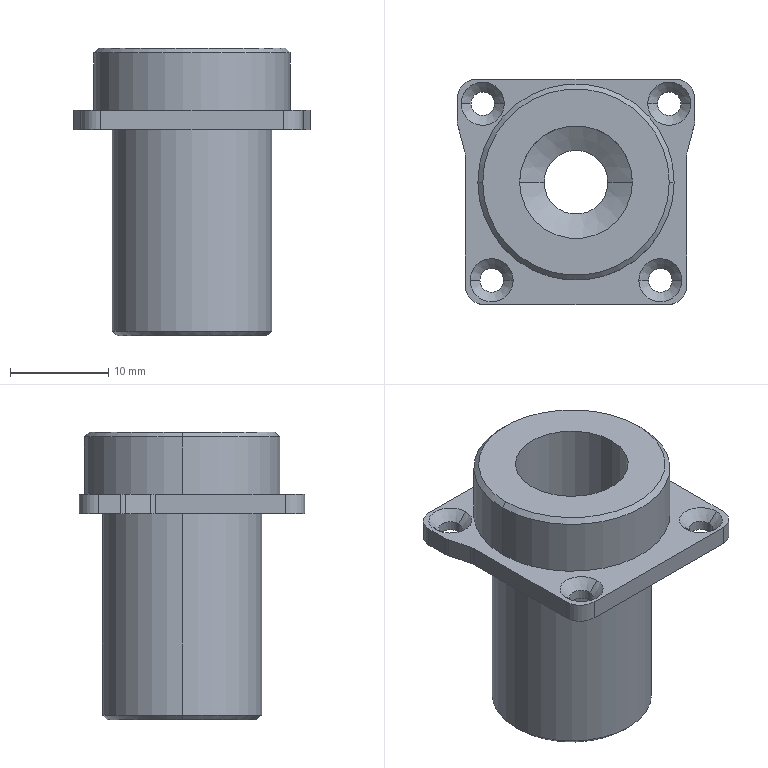NC program | NX | posted with a generic post | part box 24.2 x 23 x 29.342 mm
Lines 755 to 2259 of 2259, first 1372 of 1489 lines:
(PLANAR_MILL_4 , TOOL : D4-12-D4-50-3T-ROUGH)
N1484 T04 M6
N1486 G54
N1488 G17 G0 G90 X2.369 Y-3.011 S6500 M3
N1490 G43 Z20. H4
N1492 Z1.
N1494 G94 G1 X2.744 Y-2.744 Z0.996 F1500.
N1496 X3.485 Y-1.705 Z0.985
N1498 X3.85 Y-0.482 Z0.974
N1500 Y0.482 Z0.965
N1502 X3.485 Y1.705 Z0.954
N1504 X2.744 Y2.744 Z0.943
N1506 X1.705 Y3.485 Z0.932
N1508 X0.482 Y3.85 Z0.921
N1510 X-0.482 Z0.912
N1512 X-1.705 Y3.485 Z0.901
N1514 X-2.744 Y2.744 Z0.89
N1516 X-3.485 Y1.705 Z0.879
N1518 X-3.85 Y0.482 Z0.868
N1520 Y-0.482 Z0.859
N1522 X-3.485 Y-1.705 Z0.848
N1524 X-2.744 Y-2.744 Z0.837
N1526 X-1.705 Y-3.485 Z0.826
N1528 X-0.482 Y-3.85 Z0.815
N1530 X0.482 Z0.806
N1532 X1.705 Y-3.485 Z0.795
N1534 X2.744 Y-2.744 Z0.784
N1536 X3.485 Y-1.705 Z0.773
N1538 X3.85 Y-0.482 Z0.762
N1540 Y0.482 Z0.753
N1542 X3.485 Y1.705 Z0.742
N1544 X2.744 Y2.744 Z0.731
N1546 X1.705 Y3.485 Z0.72
N1548 X0.482 Y3.85 Z0.709
N1550 X-0.482 Z0.7
N1552 X-1.705 Y3.485 Z0.689
N1554 X-2.744 Y2.744 Z0.678
N1556 X-3.485 Y1.705 Z0.667
N1558 X-3.85 Y0.482 Z0.656
N1560 Y-0.482 Z0.648
N1562 X-3.485 Y-1.705 Z0.636
N1564 X-2.744 Y-2.744 Z0.625
N1566 X-1.705 Y-3.485 Z0.614
N1568 X-0.482 Y-3.85 Z0.603
N1570 X0.482 Z0.595
N1572 X1.705 Y-3.485 Z0.583
N1574 X2.744 Y-2.744 Z0.572
N1576 X3.485 Y-1.705 Z0.561
N1578 X3.85 Y-0.482 Z0.55
N1580 Y0.482 Z0.542
N1582 X3.485 Y1.705 Z0.53
N1584 X2.744 Y2.744 Z0.519
N1586 X1.705 Y3.485 Z0.508
N1588 X0.482 Y3.85 Z0.497
N1590 X-0.482 Z0.489
N1592 X-1.705 Y3.485 Z0.478
N1594 X-2.744 Y2.744 Z0.466
N1596 X-3.485 Y1.705 Z0.455
N1598 X-3.85 Y0.482 Z0.444
N1600 Y-0.482 Z0.436
N1602 X-3.485 Y-1.705 Z0.425
N1604 X-2.744 Y-2.744 Z0.413
N1606 X-1.705 Y-3.485 Z0.402
N1608 X-0.482 Y-3.85 Z0.391
N1610 X0.482 Z0.383
N1612 X1.705 Y-3.485 Z0.372
N1614 X2.744 Y-2.744 Z0.36
N1616 X3.485 Y-1.705 Z0.349
N1618 X3.85 Y-0.482 Z0.338
N1620 Y0.482 Z0.33
N1622 X3.485 Y1.705 Z0.319
N1624 X2.744 Y2.744 Z0.307
N1626 X1.705 Y3.485 Z0.296
N1628 X0.482 Y3.85 Z0.285
N1630 X-0.482 Z0.277
N1632 X-1.705 Y3.485 Z0.266
N1634 X-2.744 Y2.744 Z0.255
N1636 X-3.485 Y1.705 Z0.243
N1638 X-3.85 Y0.482 Z0.232
N1640 Y-0.482 Z0.224
N1642 X-3.485 Y-1.705 Z0.213
N1644 X-2.744 Y-2.744 Z0.202
N1646 X-1.705 Y-3.485 Z0.19
N1648 X-0.482 Y-3.85 Z0.179
N1650 X0.482 Z0.171
N1652 X1.705 Y-3.485 Z0.16
N1654 X2.744 Y-2.744 Z0.149
N1656 X3.485 Y-1.705 Z0.137
N1658 X3.85 Y-0.482 Z0.126
N1660 Y0.482 Z0.118
N1662 X3.485 Y1.705 Z0.107
N1664 X2.744 Y2.744 Z0.096
N1666 X1.705 Y3.485 Z0.084
N1668 X0.482 Y3.85 Z0.073
N1670 X-0.482 Z0.065
N1672 X-1.705 Y3.485 Z0.054
N1674 X-2.744 Y2.744 Z0.043
N1676 X-3.485 Y1.705 Z0.032
N1678 X-3.85 Y0.482 Z0.02
N1680 Y-0.482 Z0.012
N1682 X-3.485 Y-1.705 Z0.001
N1684 X-2.744 Y-2.744 Z-0.01
N1686 X-1.705 Y-3.485 Z-0.021
N1688 X-0.482 Y-3.85 Z-0.033
N1690 X0.482 Z-0.041
N1692 X1.705 Y-3.485 Z-0.052
N1694 X2.744 Y-2.744 Z-0.063
N1696 X3.485 Y-1.705 Z-0.074
N1698 X3.85 Y-0.482 Z-0.086
N1700 Y0.482 Z-0.094
N1702 X3.485 Y1.705 Z-0.105
N1704 X2.744 Y2.744 Z-0.116
N1706 X1.705 Y3.485 Z-0.127
N1708 X0.482 Y3.85 Z-0.139
N1710 X-0.482 Z-0.147
N1712 X-1.705 Y3.485 Z-0.158
N1714 X-2.744 Y2.744 Z-0.169
N1716 X-3.485 Y1.705 Z-0.18
N1718 X-3.85 Y0.482 Z-0.191
N1720 Y-0.482 Z-0.2
N1722 X-3.485 Y-1.705 Z-0.211
N1724 X-2.744 Y-2.744 Z-0.222
N1726 X-1.705 Y-3.485 Z-0.233
N1728 X-0.482 Y-3.85 Z-0.244
N1730 X0.482 Z-0.253
N1732 X1.705 Y-3.485 Z-0.264
N1734 X2.744 Y-2.744 Z-0.275
N1736 X3.485 Y-1.705 Z-0.286
N1738 X3.85 Y-0.482 Z-0.297
N1740 Y0.482 Z-0.306
N1742 X3.485 Y1.705 Z-0.317
N1744 X2.744 Y2.744 Z-0.328
N1746 X1.705 Y3.485 Z-0.339
N1748 X0.482 Y3.85 Z-0.35
N1750 X-0.482 Z-0.359
N1752 X-1.705 Y3.485 Z-0.37
N1754 X-2.744 Y2.744 Z-0.381
N1756 X-3.485 Y1.705 Z-0.392
N1758 X-3.85 Y0.482 Z-0.403
N1760 Y-0.482 Z-0.412
N1762 X-3.485 Y-1.705 Z-0.423
N1764 X-2.744 Y-2.744 Z-0.434
N1766 X-1.705 Y-3.485 Z-0.445
N1768 X-0.482 Y-3.85 Z-0.456
N1770 X0.482 Z-0.465
N1772 X1.705 Y-3.485 Z-0.476
N1774 X2.744 Y-2.744 Z-0.487
N1776 X3.485 Y-1.705 Z-0.498
N1778 X3.85 Y-0.482 Z-0.509
N1780 Y0.482 Z-0.518
N1782 X3.485 Y1.705 Z-0.529
N1784 X2.744 Y2.744 Z-0.54
N1786 X1.705 Y3.485 Z-0.551
N1788 X0.482 Y3.85 Z-0.562
N1790 X-0.482 Z-0.571
N1792 X-1.705 Y3.485 Z-0.582
N1794 X-2.744 Y2.744 Z-0.593
N1796 X-3.485 Y1.705 Z-0.604
N1798 X-3.85 Y0.482 Z-0.615
N1800 Y-0.482 Z-0.624
N1802 X-3.485 Y-1.705 Z-0.635
N1804 X-2.744 Y-2.744 Z-0.646
N1806 X-1.705 Y-3.485 Z-0.657
N1808 X-0.482 Y-3.85 Z-0.668
N1810 X0.482 Z-0.677
N1812 X1.705 Y-3.485 Z-0.688
N1814 X2.744 Y-2.744 Z-0.699
N1816 X3.485 Y-1.705 Z-0.71
N1818 X3.85 Y-0.482 Z-0.721
N1820 Y0.482 Z-0.729
N1822 X3.485 Y1.705 Z-0.741
N1824 X2.744 Y2.744 Z-0.752
N1826 X1.705 Y3.485 Z-0.763
N1828 X0.482 Y3.85 Z-0.774
N1830 X-0.482 Z-0.782
N1832 X-1.705 Y3.485 Z-0.794
N1834 X-2.744 Y2.744 Z-0.805
N1836 X-3.485 Y1.705 Z-0.816
N1838 X-3.85 Y0.482 Z-0.827
N1840 Y-0.482 Z-0.835
N1842 X-3.485 Y-1.705 Z-0.847
N1844 X-2.744 Y-2.744 Z-0.858
N1846 X-1.705 Y-3.485 Z-0.869
N1848 X-0.482 Y-3.85 Z-0.88
N1850 X0.482 Z-0.888
N1852 X1.705 Y-3.485 Z-0.9
N1854 X2.744 Y-2.744 Z-0.911
N1856 X3.485 Y-1.705 Z-0.922
N1858 X3.85 Y-0.482 Z-0.933
N1860 Y0.482 Z-0.941
N1862 X3.485 Y1.705 Z-0.952
N1864 X2.744 Y2.744 Z-0.964
N1866 X1.705 Y3.485 Z-0.975
N1868 X0.482 Y3.85 Z-0.986
N1870 X-0.482 Z-0.994
N1872 X-1.705 Y3.485 Z-1.005
N1874 X-2.744 Y2.744 Z-1.017
N1876 X-3.485 Y1.705 Z-1.028
N1878 X-3.85 Y0.482 Z-1.039
N1880 Y-0.482 Z-1.047
N1882 X-3.485 Y-1.705 Z-1.058
N1884 X-2.744 Y-2.744 Z-1.07
N1886 X-1.705 Y-3.485 Z-1.081
N1888 X-0.482 Y-3.85 Z-1.092
N1890 X0.482 Z-1.1
N1892 X1.705 Y-3.485 Z-1.111
N1894 X2.744 Y-2.744 Z-1.123
N1896 X3.485 Y-1.705 Z-1.134
N1898 X3.85 Y-0.482 Z-1.145
N1900 Y0.482 Z-1.153
N1902 X3.485 Y1.705 Z-1.164
N1904 X2.744 Y2.744 Z-1.175
N1906 X1.705 Y3.485 Z-1.187
N1908 X0.482 Y3.85 Z-1.198
N1910 X-0.482 Z-1.206
N1912 X-1.705 Y3.485 Z-1.217
N1914 X-2.744 Y2.744 Z-1.228
N1916 X-3.485 Y1.705 Z-1.24
N1918 X-3.85 Y0.482 Z-1.251
N1920 Y-0.482 Z-1.259
N1922 X-3.485 Y-1.705 Z-1.27
N1924 X-2.744 Y-2.744 Z-1.281
N1926 X-1.705 Y-3.485 Z-1.293
N1928 X-0.482 Y-3.85 Z-1.304
N1930 X0.482 Z-1.312
N1932 X1.705 Y-3.485 Z-1.323
N1934 X2.744 Y-2.744 Z-1.334
N1936 X3.485 Y-1.705 Z-1.346
N1938 X3.85 Y-0.482 Z-1.357
N1940 Y0.482 Z-1.365
N1942 X3.485 Y1.705 Z-1.376
N1944 X2.744 Y2.744 Z-1.387
N1946 X1.705 Y3.485 Z-1.398
N1948 X0.482 Y3.85 Z-1.41
N1950 X-0.482 Z-1.418
N1952 X-1.705 Y3.485 Z-1.429
N1954 X-2.744 Y2.744 Z-1.44
N1956 X-3.485 Y1.705 Z-1.451
N1958 X-3.85 Y0.482 Z-1.463
N1960 Y-0.482 Z-1.471
N1962 X-3.485 Y-1.705 Z-1.482
N1964 X-2.744 Y-2.744 Z-1.493
N1966 X-1.705 Y-3.485 Z-1.504
N1968 X-0.482 Y-3.85 Z-1.516
N1970 X0.482 Z-1.524
N1972 X1.705 Y-3.485 Z-1.535
N1974 X2.744 Y-2.744 Z-1.546
N1976 X3.485 Y-1.705 Z-1.557
N1978 X3.85 Y-0.482 Z-1.568
N1980 Y0.482 Z-1.577
N1982 X3.485 Y1.705 Z-1.588
N1984 X2.744 Y2.744 Z-1.599
N1986 X1.705 Y3.485 Z-1.61
N1988 X0.482 Y3.85 Z-1.621
N1990 X-0.482 Z-1.63
N1992 X-1.705 Y3.485 Z-1.641
N1994 X-2.744 Y2.744 Z-1.652
N1996 X-3.485 Y1.705 Z-1.663
N1998 X-3.85 Y0.482 Z-1.674
N2000 Y-0.482 Z-1.683
N2002 X-3.485 Y-1.705 Z-1.694
N2004 X-2.744 Y-2.744 Z-1.705
N2006 X-1.705 Y-3.485 Z-1.716
N2008 X-0.482 Y-3.85 Z-1.727
N2010 X0.482 Z-1.736
N2012 X1.705 Y-3.485 Z-1.747
N2014 X2.744 Y-2.744 Z-1.758
N2016 X3.485 Y-1.705 Z-1.769
N2018 X3.85 Y-0.482 Z-1.78
N2020 Y0.482 Z-1.789
N2022 X3.485 Y1.705 Z-1.8
N2024 X2.744 Y2.744 Z-1.811
N2026 X1.705 Y3.485 Z-1.822
N2028 X0.482 Y3.85 Z-1.833
N2030 X-0.482 Z-1.842
N2032 X-1.705 Y3.485 Z-1.853
N2034 X-2.744 Y2.744 Z-1.864
N2036 X-3.485 Y1.705 Z-1.875
N2038 X-3.85 Y0.482 Z-1.886
N2040 Y-0.482 Z-1.895
N2042 X-3.485 Y-1.705 Z-1.906
N2044 X-2.744 Y-2.744 Z-1.917
N2046 X-1.705 Y-3.485 Z-1.928
N2048 X-0.482 Y-3.85 Z-1.939
N2050 X0.482 Z-1.948
N2052 X1.705 Y-3.485 Z-1.959
N2054 X2.744 Y-2.744 Z-1.97
N2056 X3.485 Y-1.705 Z-1.981
N2058 X3.85 Y-0.482 Z-1.992
N2060 Y0.482 Z-2.001
N2062 X3.485 Y1.705 Z-2.012
N2064 X2.744 Y2.744 Z-2.023
N2066 X1.705 Y3.485 Z-2.034
N2068 X0.482 Y3.85 Z-2.045
N2070 X-0.482 Z-2.054
N2072 X-1.705 Y3.485 Z-2.065
N2074 X-2.744 Y2.744 Z-2.076
N2076 X-3.485 Y1.705 Z-2.087
N2078 X-3.85 Y0.482 Z-2.098
N2080 Y-0.482 Z-2.107
N2082 X-3.485 Y-1.705 Z-2.118
N2084 X-2.744 Y-2.744 Z-2.129
N2086 X-1.705 Y-3.485 Z-2.14
N2088 X-0.482 Y-3.85 Z-2.151
N2090 X0.482 Z-2.159
N2092 X1.705 Y-3.485 Z-2.171
N2094 X2.744 Y-2.744 Z-2.182
N2096 X3.485 Y-1.705 Z-2.193
N2098 X3.85 Y-0.482 Z-2.204
N2100 Y0.482 Z-2.212
N2102 X3.485 Y1.705 Z-2.224
N2104 X2.744 Y2.744 Z-2.235
N2106 X1.705 Y3.485 Z-2.246
N2108 X0.482 Y3.85 Z-2.257
N2110 X-0.482 Z-2.265
N2112 X-1.705 Y3.485 Z-2.277
N2114 X-2.744 Y2.744 Z-2.288
N2116 X-3.485 Y1.705 Z-2.299
N2118 X-3.85 Y0.482 Z-2.31
N2120 Y-0.482 Z-2.318
N2122 X-3.485 Y-1.705 Z-2.33
N2124 X-2.744 Y-2.744 Z-2.341
N2126 X-1.705 Y-3.485 Z-2.352
N2128 X-0.482 Y-3.85 Z-2.363
N2130 X0.482 Z-2.371
N2132 X1.705 Y-3.485 Z-2.382
N2134 X2.744 Y-2.744 Z-2.394
N2136 X3.485 Y-1.705 Z-2.405
N2138 X3.85 Y-0.482 Z-2.416
N2140 Y0.482 Z-2.424
N2142 X3.485 Y1.705 Z-2.435
N2144 X2.744 Y2.744 Z-2.447
N2146 X1.705 Y3.485 Z-2.458
N2148 X0.482 Y3.85 Z-2.469
N2150 X-0.482 Z-2.477
N2152 X-1.705 Y3.485 Z-2.488
N2154 X-2.744 Y2.744 Z-2.5
N2156 X-3.485 Y1.705 Z-2.511
N2158 X-3.85 Y0.482 Z-2.522
N2160 Y-0.482 Z-2.53
N2162 X-3.485 Y-1.705 Z-2.541
N2164 X-2.744 Y-2.744 Z-2.552
N2166 X-1.705 Y-3.485 Z-2.564
N2168 X-0.482 Y-3.85 Z-2.575
N2170 X0.482 Z-2.583
N2172 X1.705 Y-3.485 Z-2.594
N2174 X2.744 Y-2.744 Z-2.605
N2176 X3.485 Y-1.705 Z-2.617
N2178 X3.85 Y-0.482 Z-2.628
N2180 Y0.482 Z-2.636
N2182 X3.485 Y1.705 Z-2.647
N2184 X2.744 Y2.744 Z-2.658
N2186 X1.705 Y3.485 Z-2.67
N2188 X0.482 Y3.85 Z-2.681
N2190 X-0.482 Z-2.689
N2192 X-1.705 Y3.485 Z-2.7
N2194 X-2.744 Y2.744 Z-2.711
N2196 X-3.485 Y1.705 Z-2.723
N2198 X-3.85 Y0.482 Z-2.734
N2200 Y-0.482 Z-2.742
N2202 X-3.485 Y-1.705 Z-2.753
N2204 X-2.744 Y-2.744 Z-2.764
N2206 X-1.705 Y-3.485 Z-2.775
N2208 X-0.482 Y-3.85 Z-2.787
N2210 X0.482 Z-2.795
N2212 X1.705 Y-3.485 Z-2.806
N2214 X2.744 Y-2.744 Z-2.817
N2216 X3.485 Y-1.705 Z-2.828
N2218 X3.85 Y-0.482 Z-2.84
N2220 Y0.482 Z-2.848
N2222 X3.485 Y1.705 Z-2.859
N2224 X2.744 Y2.744 Z-2.87
N2226 X1.705 Y3.485 Z-2.881
N2228 X0.482 Y3.85 Z-2.893
N2230 X-0.482 Z-2.901
N2232 X-1.705 Y3.485 Z-2.912
N2234 X-2.744 Y2.744 Z-2.923
N2236 X-3.485 Y1.705 Z-2.934
N2238 X-3.85 Y0.482 Z-2.946
N2240 Y-0.482 Z-2.954
N2242 X-3.485 Y-1.705 Z-2.965
N2244 X-2.744 Y-2.744 Z-2.976
N2246 X-1.705 Y-3.485 Z-2.987
N2248 X-0.482 Y-3.85 Z-2.998
N2250 X0.482 Z-3.007
N2252 X1.705 Y-3.485 Z-3.018
N2254 X2.744 Y-2.744 Z-3.029
N2256 X3.485 Y-1.705 Z-3.04
N2258 X3.85 Y-0.482 Z-3.051
N2260 Y0.482 Z-3.06
N2262 X3.485 Y1.705 Z-3.071
N2264 X2.744 Y2.744 Z-3.082
N2266 X1.705 Y3.485 Z-3.093
N2268 X0.482 Y3.85 Z-3.104
N2270 X-0.482 Z-3.113
N2272 X-1.705 Y3.485 Z-3.124
N2274 X-2.744 Y2.744 Z-3.135
N2276 X-3.485 Y1.705 Z-3.146
N2278 X-3.85 Y0.482 Z-3.157
N2280 Y-0.482 Z-3.166
N2282 X-3.485 Y-1.705 Z-3.177
N2284 X-2.744 Y-2.744 Z-3.188
N2286 X-1.705 Y-3.485 Z-3.199
N2288 X-0.482 Y-3.85 Z-3.21
N2290 X0.482 Z-3.219
N2292 X1.705 Y-3.485 Z-3.23
N2294 X2.744 Y-2.744 Z-3.241
N2296 X3.485 Y-1.705 Z-3.252
N2298 X3.85 Y-0.482 Z-3.263
N2300 Y0.482 Z-3.272
N2302 X3.485 Y1.705 Z-3.283
N2304 X2.744 Y2.744 Z-3.294
N2306 X1.705 Y3.485 Z-3.305
N2308 X0.482 Y3.85 Z-3.316
N2310 X-0.482 Z-3.325
N2312 X-1.705 Y3.485 Z-3.336
N2314 X-2.744 Y2.744 Z-3.347
N2316 X-3.485 Y1.705 Z-3.358
N2318 X-3.85 Y0.482 Z-3.369
N2320 Y-0.482 Z-3.378
N2322 X-3.485 Y-1.705 Z-3.389
N2324 X-2.744 Y-2.744 Z-3.4
N2326 X-1.705 Y-3.485 Z-3.411
N2328 X-0.482 Y-3.85 Z-3.422
N2330 X0.482 Z-3.431
N2332 X1.705 Y-3.485 Z-3.442
N2334 X2.744 Y-2.744 Z-3.453
N2336 X3.485 Y-1.705 Z-3.464
N2338 X3.85 Y-0.482 Z-3.475
N2340 Y0.482 Z-3.484
N2342 X3.485 Y1.705 Z-3.495
N2344 X2.744 Y2.744 Z-3.506
N2346 X1.705 Y3.485 Z-3.517
N2348 X0.482 Y3.85 Z-3.528
N2350 X-0.482 Z-3.537
N2352 X-1.705 Y3.485 Z-3.548
N2354 X-2.744 Y2.744 Z-3.559
N2356 X-3.485 Y1.705 Z-3.57
N2358 X-3.85 Y0.482 Z-3.581
N2360 Y-0.482 Z-3.589
N2362 X-3.485 Y-1.705 Z-3.601
N2364 X-2.744 Y-2.744 Z-3.612
N2366 X-1.705 Y-3.485 Z-3.623
N2368 X-0.482 Y-3.85 Z-3.634
N2370 X0.482 Z-3.642
N2372 X1.705 Y-3.485 Z-3.654
N2374 X2.744 Y-2.744 Z-3.665
N2376 X3.485 Y-1.705 Z-3.676
N2378 X3.85 Y-0.482 Z-3.687
N2380 Y0.482 Z-3.695
N2382 X3.485 Y1.705 Z-3.707
N2384 X2.744 Y2.744 Z-3.718
N2386 X1.705 Y3.485 Z-3.729
N2388 X0.482 Y3.85 Z-3.74
N2390 X-0.482 Z-3.748
N2392 X-1.705 Y3.485 Z-3.759
N2394 X-2.744 Y2.744 Z-3.771
N2396 X-3.485 Y1.705 Z-3.782
N2398 X-3.85 Y0.482 Z-3.793
N2400 Y-0.482 Z-3.801
N2402 X-3.485 Y-1.705 Z-3.812
N2404 X-2.744 Y-2.744 Z-3.824
N2406 X-1.705 Y-3.485 Z-3.835
N2408 X-0.482 Y-3.85 Z-3.846
N2410 X0.482 Z-3.854
N2412 X1.705 Y-3.485 Z-3.865
N2414 X2.744 Y-2.744 Z-3.877
N2416 X3.485 Y-1.705 Z-3.888
N2418 X3.85 Y-0.482 Z-3.899
N2420 Y0.482 Z-3.907
N2422 X3.485 Y1.705 Z-3.918
N2424 X2.744 Y2.744 Z-3.93
N2426 X1.705 Y3.485 Z-3.941
N2428 X0.482 Y3.85 Z-3.952
N2430 X-0.482 Z-3.96
N2432 X-1.705 Y3.485 Z-3.971
N2434 X-2.744 Y2.744 Z-3.982
N2436 X-3.485 Y1.705 Z-3.994
N2438 X-3.85 Y0.482 Z-4.005
N2440 Y-0.482 Z-4.013
N2442 X-3.485 Y-1.705 Z-4.024
N2444 X-2.744 Y-2.744 Z-4.035
N2446 X-1.705 Y-3.485 Z-4.047
N2448 X-0.482 Y-3.85 Z-4.058
N2450 X0.482 Z-4.066
N2452 X1.705 Y-3.485 Z-4.077
N2454 X2.744 Y-2.744 Z-4.088
N2456 X3.485 Y-1.705 Z-4.1
N2458 X3.85 Y-0.482 Z-4.111
N2460 Y0.482 Z-4.119
N2462 X3.485 Y1.705 Z-4.13
N2464 X2.744 Y2.744 Z-4.141
N2466 X1.705 Y3.485 Z-4.153
N2468 X0.482 Y3.85 Z-4.164
N2470 X-0.482 Z-4.172
N2472 X-1.705 Y3.485 Z-4.183
N2474 X-2.744 Y2.744 Z-4.194
N2476 X-3.485 Y1.705 Z-4.205
N2478 X-3.85 Y0.482 Z-4.217
N2480 Y-0.482 Z-4.225
N2482 X-3.485 Y-1.705 Z-4.236
N2484 X-2.744 Y-2.744 Z-4.247
N2486 X-1.705 Y-3.485 Z-4.258
N2488 X-0.482 Y-3.85 Z-4.27
N2490 X0.482 Z-4.278
N2492 X1.705 Y-3.485 Z-4.289
N2494 X2.744 Y-2.744 Z-4.3
N2496 X3.485 Y-1.705 Z-4.311
N2498 X3.85 Y-0.482 Z-4.323
N2500 Y0.482 Z-4.331
N2502 X3.485 Y1.705 Z-4.342
N2504 X2.744 Y2.744 Z-4.353
N2506 X1.705 Y3.485 Z-4.364
N2508 X0.482 Y3.85 Z-4.375
N2510 X-0.482 Z-4.384
N2512 X-1.705 Y3.485 Z-4.395
N2514 X-2.744 Y2.744 Z-4.406
N2516 X-3.485 Y1.705 Z-4.417
N2518 X-3.85 Y0.482 Z-4.428
N2520 Y-0.482 Z-4.437
N2522 X-3.485 Y-1.705 Z-4.448
N2524 X-2.744 Y-2.744 Z-4.459
N2526 X-1.705 Y-3.485 Z-4.47
N2528 X-0.482 Y-3.85 Z-4.481
N2530 X0.482 Z-4.49
N2532 X1.705 Y-3.485 Z-4.501
N2534 X2.744 Y-2.744 Z-4.512
N2536 X3.485 Y-1.705 Z-4.523
N2538 X3.85 Y-0.482 Z-4.534
N2540 Y0.482 Z-4.543
N2542 X3.485 Y1.705 Z-4.554
N2544 X2.744 Y2.744 Z-4.565
N2546 X1.705 Y3.485 Z-4.576
N2548 X0.482 Y3.85 Z-4.587
N2550 X-0.482 Z-4.596
N2552 X-1.705 Y3.485 Z-4.607
N2554 X-2.744 Y2.744 Z-4.618
N2556 X-3.485 Y1.705 Z-4.629
N2558 X-3.85 Y0.482 Z-4.64
N2560 Y-0.482 Z-4.649
N2562 X-3.485 Y-1.705 Z-4.66
N2564 X-2.744 Y-2.744 Z-4.671
N2566 X-1.705 Y-3.485 Z-4.682
N2568 X-0.482 Y-3.85 Z-4.693
N2570 X0.482 Z-4.702
N2572 X1.705 Y-3.485 Z-4.713
N2574 X2.744 Y-2.744 Z-4.724
N2576 X3.485 Y-1.705 Z-4.735
N2578 X3.85 Y-0.482 Z-4.746
N2580 Y0.482 Z-4.755
N2582 X3.485 Y1.705 Z-4.766
N2584 X2.744 Y2.744 Z-4.777
N2586 X1.705 Y3.485 Z-4.788
N2588 X0.482 Y3.85 Z-4.799
N2590 X-0.482 Z-4.808
N2592 X-1.705 Y3.485 Z-4.819
N2594 X-2.744 Y2.744 Z-4.83
N2596 X-3.485 Y1.705 Z-4.841
N2598 X-3.85 Y0.482 Z-4.852
N2600 Y-0.482 Z-4.861
N2602 X-3.485 Y-1.705 Z-4.872
N2604 X-2.744 Y-2.744 Z-4.883
N2606 X-1.705 Y-3.485 Z-4.894
N2608 X-0.482 Y-3.85 Z-4.905
N2610 X0.482 Z-4.914
N2612 X1.705 Y-3.485 Z-4.925
N2614 X2.744 Y-2.744 Z-4.936
N2616 X3.485 Y-1.705 Z-4.947
N2618 X3.85 Y-0.482 Z-4.958
N2620 Y0.482 Z-4.966
N2622 X3.485 Y1.705 Z-4.978
N2624 X2.744 Y2.744 Z-4.989
N2626 X1.705 Y3.485 Z-5.
N2628 X0.482 Y3.85 Z-5.011
N2630 X-0.482 Z-5.019
N2632 X-1.705 Y3.485 Z-5.031
N2634 X-2.744 Y2.744 Z-5.042
N2636 X-3.485 Y1.705 Z-5.053
N2638 X-3.85 Y0.482 Z-5.064
N2640 Y-0.482 Z-5.072
N2642 X-3.485 Y-1.705 Z-5.084
N2644 X-2.744 Y-2.744 Z-5.095
N2646 X-1.705 Y-3.485 Z-5.106
N2648 X-0.482 Y-3.85 Z-5.117
N2650 X0.482 Z-5.125
N2652 X1.705 Y-3.485 Z-5.137
N2654 X2.744 Y-2.744 Z-5.148
N2656 X3.485 Y-1.705 Z-5.159
N2658 X3.85 Y-0.482 Z-5.17
N2660 Y0.482 Z-5.178
N2662 X3.485 Y1.705 Z-5.189
N2664 X2.744 Y2.744 Z-5.201
N2666 X1.705 Y3.485 Z-5.212
N2668 X0.482 Y3.85 Z-5.223
N2670 X-0.482 Z-5.231
N2672 X-1.705 Y3.485 Z-5.242
N2674 X-2.744 Y2.744 Z-5.254
N2676 X-3.485 Y1.705 Z-5.265
N2678 X-3.85 Y0.482 Z-5.276
N2680 Y-0.482 Z-5.284
N2682 X-3.485 Y-1.705 Z-5.295
N2684 X-2.744 Y-2.744 Z-5.307
N2686 X-1.705 Y-3.485 Z-5.318
N2688 X-0.482 Y-3.85 Z-5.329
N2690 X0.482 Z-5.337
N2692 X1.705 Y-3.485 Z-5.348
N2694 X2.744 Y-2.744 Z-5.36
N2696 X3.485 Y-1.705 Z-5.371
N2698 X3.85 Y-0.482 Z-5.382
N2700 Y0.482 Z-5.39
N2702 X3.485 Y1.705 Z-5.401
N2704 X2.744 Y2.744 Z-5.412
N2706 X1.705 Y3.485 Z-5.424
N2708 X0.482 Y3.85 Z-5.435
N2710 X-0.482 Z-5.443
N2712 X-1.705 Y3.485 Z-5.454
N2714 X-2.744 Y2.744 Z-5.465
N2716 X-3.485 Y1.705 Z-5.477
N2718 X-3.85 Y0.482 Z-5.488
N2720 Y-0.482 Z-5.496
N2722 X-3.485 Y-1.705 Z-5.507
N2724 X-2.744 Y-2.744 Z-5.518
N2726 X-1.705 Y-3.485 Z-5.53
N2728 X-0.482 Y-3.85 Z-5.541
N2730 X0.482 Z-5.549
N2732 X1.705 Y-3.485 Z-5.56
N2734 X2.744 Y-2.744 Z-5.571
N2736 X3.485 Y-1.705 Z-5.582
N2738 X3.85 Y-0.482 Z-5.594
N2740 Y0.482 Z-5.602
N2742 X3.485 Y1.705 Z-5.613
N2744 X2.744 Y2.744 Z-5.624
N2746 X1.705 Y3.485 Z-5.635
N2748 X0.482 Y3.85 Z-5.647
N2750 X-0.482 Z-5.655
N2752 X-1.705 Y3.485 Z-5.666
N2754 X-2.744 Y2.744 Z-5.677
N2756 X-3.485 Y1.705 Z-5.688
N2758 X-3.85 Y0.482 Z-5.7
N2760 Y-0.482 Z-5.708
N2762 X-3.485 Y-1.705 Z-5.719
N2764 X-2.744 Y-2.744 Z-5.73
N2766 X-1.705 Y-3.485 Z-5.741
N2768 X-0.482 Y-3.85 Z-5.753
N2770 X0.482 Z-5.761
N2772 X1.705 Y-3.485 Z-5.772
N2774 X2.744 Y-2.744 Z-5.783
N2776 X3.485 Y-1.705 Z-5.794
N2778 X3.85 Y-0.482 Z-5.805
N2780 Y0.482 Z-5.814
N2782 X3.485 Y1.705 Z-5.825
N2784 X2.744 Y2.744 Z-5.836
N2786 X1.705 Y3.485 Z-5.847
N2788 X0.482 Y3.85 Z-5.858
N2790 X-0.482 Z-5.867
N2792 X-1.705 Y3.485 Z-5.878
N2794 X-2.744 Y2.744 Z-5.889
N2796 X-3.485 Y1.705 Z-5.9
N2798 X-3.85 Y0.482 Z-5.911
N2800 Y-0.482 Z-5.92
N2802 X-3.485 Y-1.705 Z-5.931
N2804 X-2.744 Y-2.744 Z-5.942
N2806 X-1.705 Y-3.485 Z-5.953
N2808 X-0.482 Y-3.85 Z-5.964
N2810 X0.482 Z-5.973
N2812 X1.705 Y-3.485 Z-5.984
N2814 X2.744 Y-2.744 Z-5.995
N2816 X3.485 Y-1.705 Z-6.006
N2818 X3.85 Y-0.482 Z-6.017
N2820 Y0.482 Z-6.026
N2822 X3.485 Y1.705 Z-6.037
N2824 X2.744 Y2.744 Z-6.048
N2826 X1.705 Y3.485 Z-6.059
N2828 X0.482 Y3.85 Z-6.07
N2830 X-0.482 Z-6.079
N2832 X-1.705 Y3.485 Z-6.09
N2834 X-2.744 Y2.744 Z-6.101
N2836 X-3.485 Y1.705 Z-6.112
N2838 X-3.85 Y0.482 Z-6.123
N2840 Y-0.482 Z-6.132
N2842 X-3.485 Y-1.705 Z-6.143
N2844 X-2.744 Y-2.744 Z-6.154
N2846 X-1.705 Y-3.485 Z-6.165
N2848 X-0.482 Y-3.85 Z-6.176
N2850 X0.482 Z-6.185
N2852 X1.705 Y-3.485 Z-6.196
N2854 X2.744 Y-2.744 Z-6.207
N2856 X3.485 Y-1.705 Z-6.218
N2858 X3.85 Y-0.482 Z-6.229
N2860 Y0.482 Z-6.238
N2862 X3.485 Y1.705 Z-6.249
N2864 X2.744 Y2.744 Z-6.26
N2866 X1.705 Y3.485 Z-6.271
N2868 X0.482 Y3.85 Z-6.282
N2870 X-0.482 Z-6.291
N2872 X-1.705 Y3.485 Z-6.302
N2874 X-2.744 Y2.744 Z-6.313
N2876 X-3.485 Y1.705 Z-6.324
N2878 X-3.85 Y0.482 Z-6.335
N2880 Y-0.482 Z-6.344
N2882 X-3.485 Y-1.705 Z-6.355
N2884 X-2.744 Y-2.744 Z-6.366
N2886 X-1.705 Y-3.485 Z-6.377
N2888 X-0.482 Y-3.85 Z-6.388
N2890 X0.482 Z-6.396
N2892 X1.705 Y-3.485 Z-6.408
N2894 X2.744 Y-2.744 Z-6.419
N2896 X3.485 Y-1.705 Z-6.43
N2898 X3.85 Y-0.482 Z-6.441
N2900 Y0.482 Z-6.449
N2902 X3.485 Y1.705 Z-6.461
N2904 X2.744 Y2.744 Z-6.472
N2906 X1.705 Y3.485 Z-6.483
N2908 X0.482 Y3.85 Z-6.494
N2910 X-0.482 Z-6.502
N2912 X-1.705 Y3.485 Z-6.514
N2914 X-2.744 Y2.744 Z-6.525
N2916 X-3.485 Y1.705 Z-6.536
N2918 X-3.85 Y0.482 Z-6.547
N2920 Y-0.482 Z-6.555
N2922 X-3.485 Y-1.705 Z-6.567
N2924 X-2.744 Y-2.744 Z-6.578
N2926 X-1.705 Y-3.485 Z-6.589
N2928 X-0.482 Y-3.85 Z-6.6
N2930 X0.482 Z-6.608
N2932 X1.705 Y-3.485 Z-6.619
N2934 X2.744 Y-2.744 Z-6.631
N2936 X3.485 Y-1.705 Z-6.642
N2938 X3.85 Y-0.482 Z-6.653
N2940 Y0.482 Z-6.661
N2942 X3.485 Y1.705 Z-6.672
N2944 X2.744 Y2.744 Z-6.684
N2946 X1.705 Y3.485 Z-6.695
N2948 X0.482 Y3.85 Z-6.706
N2950 X-0.482 Z-6.714
N2952 X-1.705 Y3.485 Z-6.725
N2954 X-2.744 Y2.744 Z-6.737
N2956 X-3.485 Y1.705 Z-6.748
N2958 X-3.85 Y0.482 Z-6.759
N2960 Y-0.482 Z-6.767
N2962 X-3.485 Y-1.705 Z-6.778
N2964 X-2.744 Y-2.744 Z-6.789
N2966 X-1.705 Y-3.485 Z-6.801
N2968 X-0.482 Y-3.85 Z-6.812
N2970 X0.482 Z-6.82
N2972 X1.705 Y-3.485 Z-6.831
N2974 X2.744 Y-2.744 Z-6.842
N2976 X3.485 Y-1.705 Z-6.854
N2978 X3.85 Y-0.482 Z-6.865
N2980 Y0.482 Z-6.873
N2982 X3.485 Y1.705 Z-6.884
N2984 X2.744 Y2.744 Z-6.895
N2986 X1.705 Y3.485 Z-6.907
N2988 X0.482 Y3.85 Z-6.918
N2990 X-0.482 Z-6.926
N2992 X-1.705 Y3.485 Z-6.937
N2994 X-2.744 Y2.744 Z-6.948
N2996 X-3.485 Y1.705 Z-6.96
N2998 X-3.85 Y0.482 Z-6.971
N3000 Y-0.482 Z-6.979
N3002 X-3.485 Y-1.705 Z-6.99
N3004 X-2.744 Y-2.744 Z-7.001
N3006 X-1.705 Y-3.485 Z-7.012
N3008 X-0.482 Y-3.85 Z-7.024
N3010 X0.482 Z-7.032
N3012 X1.705 Y-3.485 Z-7.043
N3014 X2.744 Y-2.744 Z-7.054
N3016 X3.485 Y-1.705 Z-7.065
N3018 X3.85 Y-0.482 Z-7.077
N3020 Y0.482 Z-7.085
N3022 X3.485 Y1.705 Z-7.096
N3024 X2.744 Y2.744 Z-7.107
N3026 X1.705 Y3.485 Z-7.118
N3028 X0.482 Y3.85 Z-7.13
N3030 X-0.482 Z-7.138
N3032 X-1.705 Y3.485 Z-7.149
N3034 X-2.744 Y2.744 Z-7.16
N3036 X-3.485 Y1.705 Z-7.171
N3038 X-3.85 Y0.482 Z-7.183
N3040 Y-0.482 Z-7.191
N3042 X-3.485 Y-1.705 Z-7.202
N3044 X-2.744 Y-2.744 Z-7.213
N3046 X-1.705 Y-3.485 Z-7.224
N3048 X-0.482 Y-3.85 Z-7.235
N3050 X0.482 Z-7.244
N3052 X1.705 Y-3.485 Z-7.255
N3054 X2.744 Y-2.744 Z-7.266
N3056 X3.485 Y-1.705 Z-7.277
N3058 X3.85 Y-0.482 Z-7.288
N3060 Y0.482 Z-7.297
N3062 X3.485 Y1.705 Z-7.308
N3064 X2.744 Y2.744 Z-7.319
N3066 X1.705 Y3.485 Z-7.33
N3068 X0.482 Y3.85 Z-7.341
N3070 X-0.482 Z-7.35
N3072 X-1.705 Y3.485 Z-7.361
N3074 X-2.744 Y2.744 Z-7.372
N3076 X-3.485 Y1.705 Z-7.383
N3078 X-3.85 Y0.482 Z-7.394
N3080 Y-0.482 Z-7.403
N3082 X-3.485 Y-1.705 Z-7.414
N3084 X-2.744 Y-2.744 Z-7.425
N3086 X-1.705 Y-3.485 Z-7.436
N3088 X-0.482 Y-3.85 Z-7.447
N3090 X0.482 Z-7.456
N3092 X1.705 Y-3.485 Z-7.467
N3094 X2.744 Y-2.744 Z-7.478
N3096 X3.485 Y-1.705 Z-7.489
N3098 X3.85 Y-0.482 Z-7.5
N3100 Y0.482 Z-7.509
N3102 X3.485 Y1.705 Z-7.52
N3104 X2.744 Y2.744 Z-7.531
N3106 X1.705 Y3.485 Z-7.542
N3108 X0.482 Y3.85 Z-7.553
N3110 X-0.482 Z-7.562
N3112 X-1.705 Y3.485 Z-7.573
N3114 X-2.744 Y2.744 Z-7.584
N3116 X-3.485 Y1.705 Z-7.595
N3118 X-3.85 Y0.482 Z-7.606
N3120 Y-0.482 Z-7.615
N3122 X-3.485 Y-1.705 Z-7.626
N3124 X-2.744 Y-2.744 Z-7.637
N3126 X-1.705 Y-3.485 Z-7.648
N3128 X-0.482 Y-3.85 Z-7.659
N3130 X0.482 Z-7.668
N3132 X1.705 Y-3.485 Z-7.679
N3134 X2.744 Y-2.744 Z-7.69
N3136 X3.485 Y-1.705 Z-7.701
N3138 X3.85 Y-0.482 Z-7.712
N3140 Y0.482 Z-7.721
N3142 X3.485 Y1.705 Z-7.732
N3144 X2.744 Y2.744 Z-7.743
N3146 X1.705 Y3.485 Z-7.754
N3148 X0.482 Y3.85 Z-7.765
N3150 X-0.482 Z-7.773
N3152 X-1.705 Y3.485 Z-7.785
N3154 X-2.744 Y2.744 Z-7.796
N3156 X-3.485 Y1.705 Z-7.807
N3158 X-3.85 Y0.482 Z-7.818
N3160 Y-0.482 Z-7.826
N3162 X-3.485 Y-1.705 Z-7.838
N3164 X-2.744 Y-2.744 Z-7.849
N3166 X-1.705 Y-3.485 Z-7.86
N3168 X-0.482 Y-3.85 Z-7.871
N3170 X0.482 Z-7.879
N3172 X1.705 Y-3.485 Z-7.891
N3174 X2.744 Y-2.744 Z-7.902
N3176 X3.485 Y-1.705 Z-7.913
N3178 X3.85 Y-0.482 Z-7.924
N3180 Y0.482 Z-7.932
N3182 X3.485 Y1.705 Z-7.944
N3184 X2.744 Y2.744 Z-7.955
N3186 X1.705 Y3.485 Z-7.966
N3188 X0.482 Y3.85 Z-7.977
N3190 X-0.482 Z-7.985
N3192 X-1.705 Y3.485 Z-7.996
N3194 X-2.744 Y2.744 Z-8.008
N3196 X-3.485 Y1.705 Z-8.019
N3198 X-3.85 Y0.482 Z-8.03
N3200 Y-0.482 Z-8.038
N3202 X-3.485 Y-1.705 Z-8.049
N3204 X-2.744 Y-2.744 Z-8.061
N3206 X-1.705 Y-3.485 Z-8.072
N3208 X-0.482 Y-3.85 Z-8.083
N3210 X0.482 Z-8.091
N3212 X1.705 Y-3.485 Z-8.102
N3214 X2.744 Y-2.744 Z-8.114
N3216 X3.485 Y-1.705 Z-8.125
N3218 X3.85 Y-0.482 Z-8.136
N3220 Y0.482 Z-8.144
N3222 X3.485 Y1.705 Z-8.155
N3224 X2.744 Y2.744 Z-8.167
N3226 X1.705 Y3.485 Z-8.178
N3228 X0.482 Y3.85 Z-8.189
N3230 X-0.482 Z-8.197
N3232 X-1.705 Y3.485 Z-8.208
N3234 X-2.744 Y2.744 Z-8.219
N3236 X-3.485 Y1.705 Z-8.231
N3238 X-3.85 Y0.482 Z-8.242
N3240 Y-0.482 Z-8.25
N3242 X-3.485 Y-1.705 Z-8.261
N3244 X-2.744 Y-2.744 Z-8.272
N3246 X-1.705 Y-3.485 Z-8.284
N3248 X-0.482 Y-3.85 Z-8.295
N3250 X0.482 Z-8.303
N3252 X1.705 Y-3.485 Z-8.314
N3254 X2.744 Y-2.744 Z-8.325
N3256 X3.485 Y-1.705 Z-8.337
N3258 X3.85 Y-0.482 Z-8.348
N3260 Y0.482 Z-8.356
N3262 X3.485 Y1.705 Z-8.367
N3264 X2.744 Y2.744 Z-8.378
N3266 X1.705 Y3.485 Z-8.39
N3268 X0.482 Y3.85 Z-8.401
N3270 X-0.482 Z-8.409
N3272 X-1.705 Y3.485 Z-8.42
N3274 X-2.744 Y2.744 Z-8.431
N3276 X-3.485 Y1.705 Z-8.442
N3278 X-3.85 Y0.482 Z-8.454
N3280 Y-0.482 Z-8.462
N3282 X-3.485 Y-1.705 Z-8.473
N3284 X-2.744 Y-2.744 Z-8.484
N3286 X-1.705 Y-3.485 Z-8.495
N3288 X-0.482 Y-3.85 Z-8.507
N3290 X0.482 Z-8.515
N3292 X1.705 Y-3.485 Z-8.526
N3294 X2.744 Y-2.744 Z-8.537
N3296 X3.485 Y-1.705 Z-8.548
N3298 X3.85 Y-0.482 Z-8.56
N3300 Y0.482 Z-8.568
N3302 X3.485 Y1.705 Z-8.579
N3304 X2.744 Y2.744 Z-8.59
N3306 X1.705 Y3.485 Z-8.601
N3308 X0.482 Y3.85 Z-8.612
N3310 X-0.482 Z-8.621
N3312 X-1.705 Y3.485 Z-8.632
N3314 X-2.744 Y2.744 Z-8.643
N3316 X-3.485 Y1.705 Z-8.654
N3318 X-3.85 Y0.482 Z-8.665
N3320 Y-0.482 Z-8.674
N3322 X-3.485 Y-1.705 Z-8.685
N3324 X-2.744 Y-2.744 Z-8.696
N3326 X-1.705 Y-3.485 Z-8.707
N3328 X-0.482 Y-3.85 Z-8.718
N3330 X0.482 Z-8.727
N3332 X1.705 Y-3.485 Z-8.738
N3334 X2.744 Y-2.744 Z-8.749
N3336 X3.485 Y-1.705 Z-8.76
N3338 X3.85 Y-0.482 Z-8.771
N3340 Y0.482 Z-8.78
N3342 X3.485 Y1.705 Z-8.791
N3344 X2.744 Y2.744 Z-8.802
N3346 X1.705 Y3.485 Z-8.813
N3348 X0.482 Y3.85 Z-8.824
N3350 X-0.482 Z-8.833
N3352 X-1.705 Y3.485 Z-8.844
N3354 X-2.744 Y2.744 Z-8.855
N3356 X-3.485 Y1.705 Z-8.866
N3358 X-3.85 Y0.482 Z-8.877
N3360 Y-0.482 Z-8.886
N3362 X-3.485 Y-1.705 Z-8.897
N3364 X-2.744 Y-2.744 Z-8.908
N3366 X-1.705 Y-3.485 Z-8.919
N3368 X-0.482 Y-3.85 Z-8.93
N3370 X0.482 Z-8.939
N3372 X1.705 Y-3.485 Z-8.95
N3374 X2.744 Y-2.744 Z-8.961
N3376 X3.485 Y-1.705 Z-8.972
N3378 X3.85 Y-0.482 Z-8.983
N3380 Y0.482 Z-8.992
N3382 X3.485 Y1.705 Z-9.003
N3384 X2.744 Y2.744 Z-9.014
N3386 X1.705 Y3.485 Z-9.025
N3388 X0.482 Y3.85 Z-9.036
N3390 X-0.482 Z-9.045
N3392 X-1.705 Y3.485 Z-9.056
N3394 X-2.744 Y2.744 Z-9.067
N3396 X-3.485 Y1.705 Z-9.078
N3398 X-3.85 Y0.482 Z-9.089
N3400 Y-0.482 Z-9.098
N3402 X-3.485 Y-1.705 Z-9.109
N3404 X-2.744 Y-2.744 Z-9.12
N3406 X-1.705 Y-3.485 Z-9.131
N3408 X-0.482 Y-3.85 Z-9.142
N3410 X0.482 Z-9.151
N3412 X1.705 Y-3.485 Z-9.162
N3414 X2.744 Y-2.744 Z-9.173
N3416 X3.485 Y-1.705 Z-9.184
N3418 X3.85 Y-0.482 Z-9.195
N3420 Y0.482 Z-9.203
N3422 X3.485 Y1.705 Z-9.215
N3424 X2.744 Y2.744 Z-9.226
N3426 X1.705 Y3.485 Z-9.237
N3428 X0.482 Y3.85 Z-9.248
N3430 X-0.482 Z-9.256
N3432 X-1.705 Y3.485 Z-9.268
N3434 X-2.744 Y2.744 Z-9.279
N3436 X-3.485 Y1.705 Z-9.29
N3438 X-3.85 Y0.482 Z-9.301
N3440 Y-0.482 Z-9.309
N3442 X-3.485 Y-1.705 Z-9.321
N3444 X-2.744 Y-2.744 Z-9.332
N3446 X-1.705 Y-3.485 Z-9.343
N3448 X-0.482 Y-3.85 Z-9.354
N3450 X0.482 Z-9.362
N3452 X1.705 Y-3.485 Z-9.374
N3454 X2.744 Y-2.744 Z-9.385
N3456 X3.485 Y-1.705 Z-9.396
N3458 X3.85 Y-0.482 Z-9.407
N3460 Y0.482 Z-9.415
N3462 X3.485 Y1.705 Z-9.426
N3464 X2.744 Y2.744 Z-9.438
N3466 X1.705 Y3.485 Z-9.449
N3468 X0.482 Y3.85 Z-9.46
N3470 X-0.482 Z-9.468
N3472 X-1.705 Y3.485 Z-9.479
N3474 X-2.744 Y2.744 Z-9.491
N3476 X-3.485 Y1.705 Z-9.502
N3478 X-3.85 Y0.482 Z-9.513
N3480 Y-0.482 Z-9.521
N3482 X-3.485 Y-1.705 Z-9.532
N3484 X-2.744 Y-2.744 Z-9.544
N3486 X-1.705 Y-3.485 Z-9.555
N3488 X-0.482 Y-3.85 Z-9.566
N3490 X0.482 Z-9.574
N3492 X1.705 Y-3.485 Z-9.585
N3494 X2.744 Y-2.744 Z-9.596
N3496 X3.485 Y-1.705 Z-9.608
N3498 X3.85 Y-0.482 Z-9.619
N3500 Y0.482 Z-9.627
N3502 X3.485 Y1.705 Z-9.638
N3504 X2.744 Y2.744 Z-9.649
N3506 X1.705 Y3.485 Z-9.661
N3508 X0.482 Y3.85 Z-9.672
N3510 X-0.482 Z-9.68
N3512 X-1.705 Y3.485 Z-9.691
N3514 X-2.744 Y2.744 Z-9.702
N3516 X-3.485 Y1.705 Z-9.714
N3518 X-3.85 Y0.482 Z-9.725
N3520 Y-0.482 Z-9.733
N3522 X-3.485 Y-1.705 Z-9.744
N3524 X-2.744 Y-2.744 Z-9.755
N3526 X-1.705 Y-3.485 Z-9.767
N3528 X-0.482 Y-3.85 Z-9.778
N3530 X0.482 Z-9.786
N3532 X1.705 Y-3.485 Z-9.797
N3534 X2.744 Y-2.744 Z-9.808
N3536 X3.485 Y-1.705 Z-9.819
N3538 X3.85 Y-0.482 Z-9.831
N3540 Y0.482 Z-9.839
N3542 X3.485 Y1.705 Z-9.85
N3544 X2.744 Y2.744 Z-9.861
N3546 X1.705 Y3.485 Z-9.872
N3548 X0.482 Y3.85 Z-9.884
N3550 X-0.482 Z-9.892
N3552 X-1.705 Y3.485 Z-9.903
N3554 X-2.744 Y2.744 Z-9.914
N3556 X-3.485 Y1.705 Z-9.925
N3558 X-3.85 Y0.482 Z-9.937
N3560 Y-0.482 Z-9.945
N3562 X-3.485 Y-1.705 Z-9.956
N3564 X-2.744 Y-2.744 Z-9.967
N3566 X-1.705 Y-3.485 Z-9.978
N3568 X-0.482 Y-3.85 Z-9.99
N3570 X0.482 Z-9.998
N3572 X1.705 Y-3.485 Z-10.009
N3574 X2.744 Y-2.744 Z-10.02
N3576 X3.485 Y-1.705 Z-10.031
N3578 X3.85 Y-0.482 Z-10.042
N3580 Y0.482 Z-10.051
N3582 X3.485 Y1.705 Z-10.062
N3584 X2.744 Y2.744 Z-10.073
N3586 X1.705 Y3.485 Z-10.084
N3588 X0.482 Y3.85 Z-10.095
N3590 X-0.482 Z-10.104
N3592 X-1.705 Y3.485 Z-10.115
N3594 X-2.744 Y2.744 Z-10.126
N3596 X-3.485 Y1.705 Z-10.137
N3598 X-3.85 Y0.482 Z-10.148
N3600 Y-0.482 Z-10.157
N3602 X-3.485 Y-1.705 Z-10.168
N3604 X-2.744 Y-2.744 Z-10.179
N3606 X-1.705 Y-3.485 Z-10.19
N3608 X-0.482 Y-3.85 Z-10.201
N3610 X0.482 Z-10.21
N3612 X1.705 Y-3.485 Z-10.221
N3614 X2.744 Y-2.744 Z-10.232
N3616 X3.485 Y-1.705 Z-10.243
N3618 X3.85 Y-0.482 Z-10.254
N3620 Y0.482 Z-10.263
N3622 X3.485 Y1.705 Z-10.274
N3624 X2.744 Y2.744 Z-10.285
N3626 X1.705 Y3.485 Z-10.296
N3628 X0.482 Y3.85 Z-10.307
N3630 X-0.482 Z-10.316
N3632 X-1.705 Y3.485 Z-10.327
N3634 X-2.744 Y2.744 Z-10.338
N3636 X-3.485 Y1.705 Z-10.349
N3638 X-3.85 Y0.482 Z-10.36
N3640 Y-0.482 Z-10.369
N3642 X-3.485 Y-1.705 Z-10.38
N3644 X-2.744 Y-2.744 Z-10.391
N3646 X-1.705 Y-3.485 Z-10.402
N3648 X-0.482 Y-3.85 Z-10.413
N3650 X0.482 Z-10.422
N3652 X1.705 Y-3.485 Z-10.433
N3654 X2.744 Y-2.744 Z-10.444
N3656 X3.485 Y-1.705 Z-10.455
N3658 X3.85 Y-0.482 Z-10.466
N3660 Y0.482 Z-10.475
N3662 X3.485 Y1.705 Z-10.486
N3664 X2.744 Y2.744 Z-10.497
N3666 X1.705 Y3.485 Z-10.508
N3668 X0.482 Y3.85 Z-10.519
N3670 X-0.482 Z-10.528
N3672 X-1.705 Y3.485 Z-10.539
N3674 X-2.744 Y2.744 Z-10.55
N3676 X-3.485 Y1.705 Z-10.561
N3678 X-3.85 Y0.482 Z-10.572
N3680 Y-0.482 Z-10.581
N3682 X-3.485 Y-1.705 Z-10.592
N3684 X-2.744 Y-2.744 Z-10.603
N3686 X-1.705 Y-3.485 Z-10.614
N3688 X-0.482 Y-3.85 Z-10.625
N3690 X0.482 Z-10.633
N3692 X1.705 Y-3.485 Z-10.645
N3694 X2.744 Y-2.744 Z-10.656
N3696 X3.485 Y-1.705 Z-10.667
N3698 X3.85 Y-0.482 Z-10.678
N3700 Y0.482 Z-10.686
N3702 X3.485 Y1.705 Z-10.698
N3704 X2.744 Y2.744 Z-10.709
N3706 X1.705 Y3.485 Z-10.72
N3708 X0.482 Y3.85 Z-10.731
N3710 X-0.482 Z-10.739
N3712 X-1.705 Y3.485 Z-10.751
N3714 X-2.744 Y2.744 Z-10.762
N3716 X-3.485 Y1.705 Z-10.773
N3718 X-3.85 Y0.482 Z-10.784
N3720 Y-0.482 Z-10.792
N3722 X-3.485 Y-1.705 Z-10.803
N3724 X-2.744 Y-2.744 Z-10.815
N3726 X-1.705 Y-3.485 Z-10.826
N3728 X-0.482 Y-3.85 Z-10.837
N3730 X0.482 Z-10.845
N3732 X1.705 Y-3.485 Z-10.856
N3734 X2.744 Y-2.744 Z-10.868
N3736 X3.485 Y-1.705 Z-10.879
N3738 X3.85 Y-0.482 Z-10.89
N3740 Y0.482 Z-10.898
N3742 X3.485 Y1.705 Z-10.909
N3744 X2.744 Y2.744 Z-10.921
N3746 X1.705 Y3.485 Z-10.932
N3748 X0.482 Y3.85 Z-10.943
N3750 X-0.482 Z-10.951
N3752 X-1.705 Y3.485 Z-10.962
N3754 X-2.744 Y2.744 Z-10.974
N3756 X-3.485 Y1.705 Z-10.985
N3758 X-3.85 Y0.482 Z-10.996
N3760 Y0. Z-11.
N3762 G3 X0. Y-3.85 R3.85
N3764 X-3.85 Y0. R-3.85
N3766 G1 Z-10.
N3768 G0 Z20.
(ZLEVEL_PROFILE_STEEP , TOOL : D4-12-D4-50-3T-ROUGH)
N3770 X-2.475 Y1. S5500
N3772 Z-10.139
N3774 G1 Z-11.139 F2000.
N3776 X-2.669
N3778 G3 X-3.669 Y0. R1.
N3780 G1 Y-0.009
N3782 G3 X0.009 Y-3.669 R3.669
N3784 X-3.669 Y0. R-3.669
N3786 G1 X-3.647 Y-0.137 Z-11.151
N3788 X-3.619 Y-0.274 Z-11.163
N3790 X-3.586 Y-0.407 Z-11.175
N3792 X-3.548 Y-0.54 Z-11.187
N3794 G3 X-3.589 Y0. R-3.589
N3796 G1 X-3.566 Y-0.137 Z-11.199
N3798 X-3.538 Y-0.274 Z-11.211
N3800 X-3.505 Y-0.407 Z-11.223
N3802 X-3.466 Y-0.539 Z-11.235
N3804 G3 X-3.508 Y0. R-3.508
N3806 G1 X-3.485 Y-0.137 Z-11.248
N3808 X-3.457 Y-0.273 Z-11.26
N3810 X-3.424 Y-0.406 Z-11.272
N3812 X-3.385 Y-0.539 Z-11.284
N3814 G3 X-3.427 Y0. R-3.427
N3816 G1 X-3.405 Y-0.137 Z-11.296
N3818 X-3.376 Y-0.273 Z-11.308
N3820 X-3.342 Y-0.406 Z-11.32
N3822 X-3.303 Y-0.538 Z-11.332
N3824 G3 X-3.347 Y0. R-3.347
N3826 G1 X-3.324 Y-0.137 Z-11.345
N3828 X-3.295 Y-0.273 Z-11.357
N3830 X-3.261 Y-0.406 Z-11.369
N3832 X-3.222 Y-0.538 Z-11.381
N3834 G3 X-3.266 Y0. R-3.266
N3836 G1 X-3.243 Y-0.137 Z-11.393
N3838 X-3.214 Y-0.273 Z-11.405
N3840 X-3.18 Y-0.406 Z-11.417
N3842 X-3.14 Y-0.538 Z-11.429
N3844 G3 X-3.185 Y0. R-3.185
N3846 G1 X-3.162 Y-0.137 Z-11.441
N3848 X-3.133 Y-0.273 Z-11.454
N3850 X-3.099 Y-0.405 Z-11.466
N3852 X-3.058 Y-0.537 Z-11.478
N3854 G3 X-3.105 Y0. R-3.105
N3856 G1 X-3.082 Y-0.137 Z-11.49
N3858 X-3.052 Y-0.273 Z-11.502
N3860 X-3.017 Y-0.405 Z-11.514
N3862 X-2.976 Y-0.537 Z-11.526
N3864 G3 X-3.024 Y0. R-3.024
N3866 G1 X-3.001 Y-0.137 Z-11.538
N3868 X-2.971 Y-0.273 Z-11.55
N3870 X-2.936 Y-0.405 Z-11.563
N3872 X-2.894 Y-0.536 Z-11.575
N3874 G3 X-2.944 Y0. R-2.944
N3876 G1 X-2.92 Y-0.137 Z-11.587
N3878 X-2.89 Y-0.273 Z-11.599
N3880 X-2.855 Y-0.405 Z-11.611
N3882 X-2.812 Y-0.536 Z-11.623
N3884 G3 X-2.863 Y0. R-2.863
N3886 G1 X-2.839 Y-0.136 Z-11.635
N3888 X-2.809 Y-0.273 Z-11.647
N3890 X-2.773 Y-0.404 Z-11.659
N3892 X-2.73 Y-0.535 Z-11.672
N3894 G3 X-2.782 Y0. R-2.782
N3896 G1 X-2.759 Y-0.136 Z-11.684
N3898 X-2.728 Y-0.272 Z-11.696
N3900 X-2.692 Y-0.404 Z-11.708
N3902 X-2.648 Y-0.534 Z-11.72
N3904 G3 X-2.702 Y0. R-2.702
N3906 G1 X-2.678 Y-0.136 Z-11.732
N3908 X-2.647 Y-0.272 Z-11.744
N3910 X-2.61 Y-0.403 Z-11.756
N3912 X-2.566 Y-0.534 Z-11.769
N3914 G3 X-2.621 Y0. R-2.621
N3916 G1 X-2.597 Y-0.136 Z-11.781
N3918 X-2.566 Y-0.272 Z-11.793
N3920 X-2.529 Y-0.403 Z-11.805
N3922 X-2.484 Y-0.533 Z-11.817
N3924 G3 X-2.54 Y0. R-2.54
N3926 G1 X-2.516 Y-0.136 Z-11.829
N3928 X-2.485 Y-0.272 Z-11.841
N3930 X-2.447 Y-0.403 Z-11.853
N3932 X-2.401 Y-0.532 Z-11.865
N3934 G3 X-2.46 Y0. R-2.46
N3936 G1 X-2.443 Y-0.099 Z-11.874
N3938 X-2.404 Y-0.272 Z-11.89
N3940 X-2.365 Y-0.402 Z-11.902
N3942 X-2.319 Y-0.531 Z-11.914
N3944 G3 X-2.379 Y0. R-2.379
N3946 G1 X-2.362 Y-0.101 Z-11.923
N3948 X-2.323 Y-0.272 Z-11.938
N3950 X-2.283 Y-0.402 Z-11.95
N3952 X-2.236 Y-0.53 Z-11.962
N3954 G3 X-2.298 Y0. R-2.298
N3956 G1 X-2.281 Y-0.102 Z-11.971
N3958 X-2.242 Y-0.271 Z-11.987
N3960 X-2.202 Y-0.401 Z-11.999
N3962 X-2.154 Y-0.529 Z-12.011
N3964 G3 X-2.218 Y0. R-2.218
N3966 G1 X-2.2 Y-0.104 Z-12.02
N3968 X-2.16 Y-0.271 Z-12.035
N3970 X-2.12 Y-0.4 Z-12.047
N3972 X-2.071 Y-0.528 Z-12.059
N3974 G3 X-2.137 Y0. R-2.137
N3976 G1 X-2.119 Y-0.106 Z-12.069
N3978 X-2.079 Y-0.271 Z-12.083
N3980 X-2.038 Y-0.4 Z-12.096
N3982 X-1.988 Y-0.527 Z-12.108
N3984 G3 X-2.056 Y0. R-2.056
N3986 G1 X-2.038 Y-0.107 Z-12.117
N3988 X-1.998 Y-0.271 Z-12.132
N3990 X-1.956 Y-0.399 Z-12.144
N3992 X-1.905 Y-0.526 Z-12.156
N3994 G3 X-1.976 Y0. R-1.976
N3996 G1 X-1.957 Y-0.109 Z-12.166
N3998 X-1.917 Y-0.27 Z-12.18
N4000 X-1.873 Y-0.398 Z-12.193
N4002 X-1.821 Y-0.524 Z-12.205
N4004 G3 X-1.895 Y0. R-1.895
N4006 G1 X-1.876 Y-0.111 Z-12.214
N4008 X-1.835 Y-0.27 Z-12.229
N4010 X-1.791 Y-0.397 Z-12.241
N4012 X-1.738 Y-0.523 Z-12.253
N4014 G3 X-1.815 Y0. R-1.815
N4016 G1 X-1.794 Y-0.112 Z-12.263
N4018 X-1.754 Y-0.27 Z-12.277
N4020 X-1.709 Y-0.397 Z-12.289
N4022 X-1.654 Y-0.521 Z-12.302
N4024 G3 X-1.734 Y0. R-1.734
N4026 G1 X-1.713 Y-0.114 Z-12.312
N4028 X-1.672 Y-0.269 Z-12.326
N4030 X-1.626 Y-0.396 Z-12.338
N4032 X-1.57 Y-0.519 Z-12.35
N4034 G3 X-1.653 Y0. R-1.653
N4036 G1 X-1.632 Y-0.116 Z-12.36
N4038 X-1.59 Y-0.269 Z-12.374
N4040 X-1.543 Y-0.394 Z-12.386
N4042 X-1.485 Y-0.517 Z-12.398
N4044 G3 X-1.573 Y0. R-1.573
N4046 G1 X-1.551 Y-0.118 Z-12.409
N4048 X-1.509 Y-0.268 Z-12.423
N4050 X-1.46 Y-0.393 Z-12.435
N4052 X-1.4 Y-0.515 Z-12.447
N4054 G3 X-1.492 Y0. R-1.492
N4056 G1 X-1.469 Y-0.12 Z-12.458
N4058 X-1.427 Y-0.268 Z-12.471
N4060 X-1.377 Y-0.392 Z-12.483
N4062 X-1.315 Y-0.512 Z-12.495
N4064 G3 X-1.411 Y0. R-1.411
N4066 G1 X-1.388 Y-0.122 Z-12.506
N4068 X-1.345 Y-0.267 Z-12.52
N4070 X-1.293 Y-0.39 Z-12.532
N4072 X-1.229 Y-0.509 Z-12.544
N4074 G3 X-1.331 Y0. R-1.331
N4076 G1 X-1.306 Y-0.124 Z-12.555
N4078 X-1.262 Y-0.267 Z-12.568
N4080 X-1.209 Y-0.388 Z-12.58
N4082 X-1.143 Y-0.505 Z-12.592
N4084 G3 X-0.466 Y-1.16 R1.25
N4086 G1 X-0.072 Y-1.248
N4088 X0.072
N4090 X0.466 Y-1.16
N4092 X0.491 Y-1.149
N4094 G3 X1.149 Y-0.491 R1.25
N4096 X1.234 Y-0.202 R1.25
N4098 G1 X1.25 Y-0.001
N4100 X1.234 Y0.202
N4102 G3 X1.149 Y0.491 R1.25
N4104 X0.466 Y1.16 R1.25
N4106 G1 X0.072 Y1.248
N4108 X-0.072
N4110 X-0.144 Y1.242
N4112 X-0.438 Y1.171
N4114 X-0.491 Y1.149
N4116 G3 X-1.149 Y0.491 R1.25
N4118 X-1.234 Y0.202 R1.25
N4120 G1 X-1.25 Y0.001
N4122 X-1.234 Y-0.202
N4124 G3 X-1.143 Y-0.505 R1.25
N4126 X0.176 Y-1.016 R1.
N4128 G1 X0.003 Y-0.239
N4130 Z-11.592
N4132 G0 Z20.
N4134 M5
(DRILLING_2 , TOOL : 倒角D4-90度)
N4136 T05 M6
N4138 G54
N4140 G17 G0 G90 X-9.5 Y8. S3000 M3
N4142 G43 Z20. H5
N4144 G94 G81 G98 Z-7.642 F200. R-3.342
N4146 X9.5
N4148 X8.6 Y-10.
N4150 X-8.6
N4152 G80
N4154 G0 X-8.6 Y-10. Z20.
(PLANAR_MILL_5 , TOOL : 倒角D4-90度)
N4156 X-3.666 Y1. S4500
N4158 Z0.5
N4160 G1 Z-1.5 F800.
N4162 X-3.8
N4164 G3 X-4.8 Y0. R1.
N4166 X0. Y-4.8 R4.8
N4168 X-4.8 Y0. R-4.8
N4170 X-3.8 Y-1. R1.
N4172 G1 X-3.85 Y1.
N4174 G3 X-4.85 Y0. R1.
N4176 X0. Y-4.85 R4.85
N4178 X-4.85 Y0. R-4.85
N4180 X-3.85 Y-1. R1.
N4182 G1 X-3.718
N4184 Z0.5
N4186 G0 Z20.
(PLANAR_MILL_5_COPY , TOOL : 倒角D4-90度)
N4188 X-12.15
N4190 Z0.5
N4192 G1 Z-1.5
N4194 G3 X-11.15 Y0. R1.
N4196 G2 X0. Y11.15 R11.15
N4198 X-11.15 Y0. R-11.15
N4200 G3 X-12.15 Y1. R1.
N4202 G1 X-12.1 Y-1.
N4204 G3 X-11.1 Y0. R1.
N4206 G2 X0. Y11.1 R11.1
N4208 X-11.1 Y0. R-11.1
N4210 G3 X-12.109 Y1. R1.
N4212 G1 Z0.5
N4214 G0 Z20.
(PLANAR_MILL_6 , TOOL : 倒角D4-90度)